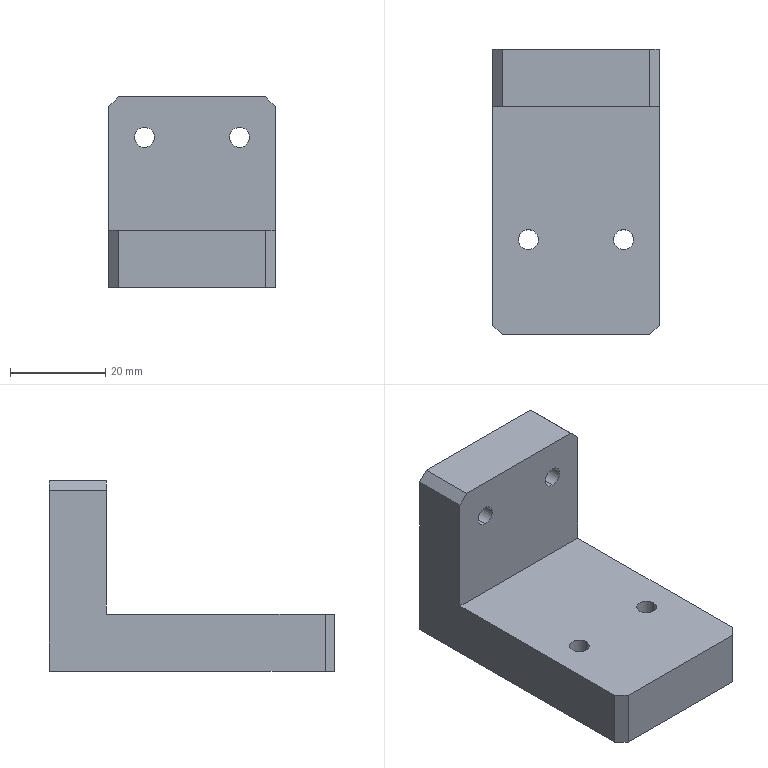Part | SolidWorks | features Chamfer 2, HoleWzd 2, Extrusion 1, ICE 1 | 1 solid | 28 faces | box 35 x 60 x 40 mm | volume 35844 mm3 | cylinder 12 | plane 12 | cone 4 | commonest cylinder face diameters 4.2 x12
STEP:
#1=CARTESIAN_POINT('',(-10.,17.6,4.4));
#2=VERTEX_POINT('',#1);
#3=CARTESIAN_POINT('',(-10.,17.6,8.6));
#4=VERTEX_POINT('',#3);
#5=CARTESIAN_POINT('',(-10.,17.6,6.5));
#6=DIRECTION('',(0.,1.,0.));
#7=DIRECTION('',(0.,0.,1.));
#8=AXIS2_PLACEMENT_3D('',#5,#6,#7);
#9=CIRCLE('',#8,2.1);
#10=EDGE_CURVE('',#2,#4,#9,.T.);
#11=ORIENTED_EDGE('',*,*,#10,.F.);
#12=CARTESIAN_POINT('',(-10.,30.,4.4));
#13=VERTEX_POINT('',#12);
#14=CARTESIAN_POINT('',(-10.,30.,4.4));
#15=DIRECTION('',(0.,1.,0.));
#16=VECTOR('',#15,1000.);
#17=LINE('',#14,#16);
#18=EDGE_CURVE('',#2,#13,#17,.T.);
#19=ORIENTED_EDGE('',*,*,#18,.T.);
#20=CARTESIAN_POINT('',(-10.,30.,8.6));
#21=VERTEX_POINT('',#20);
#22=CARTESIAN_POINT('',(-10.,30.,6.5));
#23=DIRECTION('',(0.,1.,0.));
#24=DIRECTION('',(0.,0.,1.));
#25=AXIS2_PLACEMENT_3D('',#22,#23,#24);
#26=CIRCLE('',#25,2.1);
#27=EDGE_CURVE('',#13,#21,#26,.T.);
#28=ORIENTED_EDGE('',*,*,#27,.T.);
#29=CARTESIAN_POINT('',(-10.,30.,8.6));
#30=DIRECTION('',(0.,1.,0.));
#31=VECTOR('',#30,1000.);
#32=LINE('',#29,#31);
#33=EDGE_CURVE('',#4,#21,#32,.T.);
#34=ORIENTED_EDGE('',*,*,#33,.F.);
#35=EDGE_LOOP('',(#11,#19,#28,#34));
#36=FACE_OUTER_BOUND('',#35,.T.);
#37=CARTESIAN_POINT('',(-10.,30.,6.5));
#38=DIRECTION('',(0.,1.,0.));
#39=DIRECTION('',(0.,0.,1.));
#40=AXIS2_PLACEMENT_3D('',#37,#38,#39);
#41=CYLINDRICAL_SURFACE('',#40,2.1);
#42=ADVANCED_FACE('',(#36),#41,.F.);
#43=CARTESIAN_POINT('',(-10.,16.338,6.5));
#44=VERTEX_POINT('',#43);
#45=CARTESIAN_POINT('',(-10.,17.6,8.6));
#46=DIRECTION('',(0.,0.515,0.8572));
#47=VECTOR('',#46,1000.);
#48=LINE('',#45,#47);
#49=EDGE_CURVE('',#44,#4,#48,.T.);
#50=ORIENTED_EDGE('',*,*,#49,.F.);
#51=CARTESIAN_POINT('',(-10.,17.6,4.4));
#52=DIRECTION('',(0.,0.515,-0.8572));
#53=VECTOR('',#52,1000.);
#54=LINE('',#51,#53);
#55=EDGE_CURVE('',#44,#2,#54,.T.);
#56=ORIENTED_EDGE('',*,*,#55,.T.);
#57=ORIENTED_EDGE('',*,*,#10,.T.);
#58=EDGE_LOOP('',(#50,#56,#57));
#59=FACE_OUTER_BOUND('',#58,.T.);
#60=CARTESIAN_POINT('',(-10.,17.6,6.5));
#61=DIRECTION('',(0.,1.,0.));
#62=DIRECTION('',(0.,0.,1.));
#63=AXIS2_PLACEMENT_3D('',#60,#61,#62);
#64=CONICAL_SURFACE('',#63,2.1,1.03);
#65=ADVANCED_FACE('',(#59),#64,.F.);
#66=CARTESIAN_POINT('',(10.,17.6,4.4));
#67=VERTEX_POINT('',#66);
#68=CARTESIAN_POINT('',(10.,17.6,8.6));
#69=VERTEX_POINT('',#68);
#70=CARTESIAN_POINT('',(10.,17.6,6.5));
#71=DIRECTION('',(0.,1.,0.));
#72=DIRECTION('',(0.,0.,1.));
#73=AXIS2_PLACEMENT_3D('',#70,#71,#72);
#74=CIRCLE('',#73,2.1);
#75=EDGE_CURVE('',#67,#69,#74,.T.);
#76=ORIENTED_EDGE('',*,*,#75,.F.);
#77=CARTESIAN_POINT('',(10.,30.,4.4));
#78=VERTEX_POINT('',#77);
#79=CARTESIAN_POINT('',(10.,30.,4.4));
#80=DIRECTION('',(0.,1.,0.));
#81=VECTOR('',#80,1000.);
#82=LINE('',#79,#81);
#83=EDGE_CURVE('',#67,#78,#82,.T.);
#84=ORIENTED_EDGE('',*,*,#83,.T.);
#85=CARTESIAN_POINT('',(10.,30.,8.6));
#86=VERTEX_POINT('',#85);
#87=CARTESIAN_POINT('',(10.,30.,6.5));
#88=DIRECTION('',(0.,1.,0.));
#89=DIRECTION('',(0.,0.,1.));
#90=AXIS2_PLACEMENT_3D('',#87,#88,#89);
#91=CIRCLE('',#90,2.1);
#92=EDGE_CURVE('',#78,#86,#91,.T.);
#93=ORIENTED_EDGE('',*,*,#92,.T.);
#94=CARTESIAN_POINT('',(10.,30.,8.6));
#95=DIRECTION('',(0.,1.,0.));
#96=VECTOR('',#95,1000.);
#97=LINE('',#94,#96);
#98=EDGE_CURVE('',#69,#86,#97,.T.);
#99=ORIENTED_EDGE('',*,*,#98,.F.);
#100=EDGE_LOOP('',(#76,#84,#93,#99));
#101=FACE_OUTER_BOUND('',#100,.T.);
#102=CARTESIAN_POINT('',(10.,30.,6.5));
#103=DIRECTION('',(0.,1.,0.));
#104=DIRECTION('',(0.,0.,1.));
#105=AXIS2_PLACEMENT_3D('',#102,#103,#104);
#106=CYLINDRICAL_SURFACE('',#105,2.1);
#107=ADVANCED_FACE('',(#101),#106,.F.);
#108=CARTESIAN_POINT('',(10.,16.338,6.5));
#109=VERTEX_POINT('',#108);
#110=CARTESIAN_POINT('',(10.,17.6,8.6));
#111=DIRECTION('',(0.,0.515,0.8572));
#112=VECTOR('',#111,1000.);
#113=LINE('',#110,#112);
#114=EDGE_CURVE('',#109,#69,#113,.T.);
#115=ORIENTED_EDGE('',*,*,#114,.F.);
#116=CARTESIAN_POINT('',(10.,17.6,4.4));
#117=DIRECTION('',(0.,0.515,-0.8572));
#118=VECTOR('',#117,1000.);
#119=LINE('',#116,#118);
#120=EDGE_CURVE('',#109,#67,#119,.T.);
#121=ORIENTED_EDGE('',*,*,#120,.T.);
#122=ORIENTED_EDGE('',*,*,#75,.T.);
#123=EDGE_LOOP('',(#115,#121,#122));
#124=FACE_OUTER_BOUND('',#123,.T.);
#125=CARTESIAN_POINT('',(10.,17.6,6.5));
#126=DIRECTION('',(0.,1.,0.));
#127=DIRECTION('',(0.,0.,1.));
#128=AXIS2_PLACEMENT_3D('',#125,#126,#127);
#129=CONICAL_SURFACE('',#128,2.1,1.03);
#130=ADVANCED_FACE('',(#124),#129,.F.);
#131=CARTESIAN_POINT('',(-10.,18.,33.6));
#132=VERTEX_POINT('',#131);
#133=CARTESIAN_POINT('',(-10.,18.,29.4));
#134=VERTEX_POINT('',#133);
#135=CARTESIAN_POINT('',(-10.,18.,31.5));
#136=DIRECTION('',(0.,-1.,0.));
#137=DIRECTION('',(0.,0.,-1.));
#138=AXIS2_PLACEMENT_3D('',#135,#136,#137);
#139=CIRCLE('',#138,2.1);
#140=EDGE_CURVE('',#132,#134,#139,.T.);
#141=ORIENTED_EDGE('',*,*,#140,.T.);
#142=CARTESIAN_POINT('',(-10.,30.,29.4));
#143=VERTEX_POINT('',#142);
#144=CARTESIAN_POINT('',(-10.,30.,29.4));
#145=DIRECTION('',(0.,1.,0.));
#146=VECTOR('',#145,1000.);
#147=LINE('',#144,#146);
#148=EDGE_CURVE('',#134,#143,#147,.T.);
#149=ORIENTED_EDGE('',*,*,#148,.T.);
#150=CARTESIAN_POINT('',(-10.,30.,33.6));
#151=VERTEX_POINT('',#150);
#152=CARTESIAN_POINT('',(-10.,30.,31.5));
#153=DIRECTION('',(0.,1.,0.));
#154=DIRECTION('',(0.,0.,1.));
#155=AXIS2_PLACEMENT_3D('',#152,#153,#154);
#156=CIRCLE('',#155,2.1);
#157=EDGE_CURVE('',#143,#151,#156,.T.);
#158=ORIENTED_EDGE('',*,*,#157,.T.);
#159=CARTESIAN_POINT('',(-10.,30.,33.6));
#160=DIRECTION('',(0.,1.,0.));
#161=VECTOR('',#160,1000.);
#162=LINE('',#159,#161);
#163=EDGE_CURVE('',#132,#151,#162,.T.);
#164=ORIENTED_EDGE('',*,*,#163,.F.);
#165=EDGE_LOOP('',(#141,#149,#158,#164));
#166=FACE_OUTER_BOUND('',#165,.T.);
#167=CARTESIAN_POINT('',(-10.,30.,31.5));
#168=DIRECTION('',(0.,1.,0.));
#169=DIRECTION('',(0.,0.,1.));
#170=AXIS2_PLACEMENT_3D('',#167,#168,#169);
#171=CYLINDRICAL_SURFACE('',#170,2.1);
#172=ADVANCED_FACE('',(#166),#171,.F.);
#173=CARTESIAN_POINT('',(10.,18.,33.6));
#174=VERTEX_POINT('',#173);
#175=CARTESIAN_POINT('',(10.,18.,29.4));
#176=VERTEX_POINT('',#175);
#177=CARTESIAN_POINT('',(10.,18.,31.5));
#178=DIRECTION('',(0.,-1.,0.));
#179=DIRECTION('',(0.,0.,-1.));
#180=AXIS2_PLACEMENT_3D('',#177,#178,#179);
#181=CIRCLE('',#180,2.1);
#182=EDGE_CURVE('',#174,#176,#181,.T.);
#183=ORIENTED_EDGE('',*,*,#182,.T.);
#184=CARTESIAN_POINT('',(10.,30.,29.4));
#185=VERTEX_POINT('',#184);
#186=CARTESIAN_POINT('',(10.,30.,29.4));
#187=DIRECTION('',(0.,1.,0.));
#188=VECTOR('',#187,1000.);
#189=LINE('',#186,#188);
#190=EDGE_CURVE('',#176,#185,#189,.T.);
#191=ORIENTED_EDGE('',*,*,#190,.T.);
#192=CARTESIAN_POINT('',(10.,30.,33.6));
#193=VERTEX_POINT('',#192);
#194=CARTESIAN_POINT('',(10.,30.,31.5));
#195=DIRECTION('',(0.,1.,0.));
#196=DIRECTION('',(0.,0.,1.));
#197=AXIS2_PLACEMENT_3D('',#194,#195,#196);
#198=CIRCLE('',#197,2.1);
#199=EDGE_CURVE('',#185,#193,#198,.T.);
#200=ORIENTED_EDGE('',*,*,#199,.T.);
#201=CARTESIAN_POINT('',(10.,30.,33.6));
#202=DIRECTION('',(0.,1.,0.));
#203=VECTOR('',#202,1000.);
#204=LINE('',#201,#203);
#205=EDGE_CURVE('',#174,#193,#204,.T.);
#206=ORIENTED_EDGE('',*,*,#205,.F.);
#207=EDGE_LOOP('',(#183,#191,#200,#206));
#208=FACE_OUTER_BOUND('',#207,.T.);
#209=CARTESIAN_POINT('',(10.,30.,31.5));
#210=DIRECTION('',(0.,1.,0.));
#211=DIRECTION('',(0.,0.,1.));
#212=AXIS2_PLACEMENT_3D('',#209,#210,#211);
#213=CYLINDRICAL_SURFACE('',#212,2.1);
#214=ADVANCED_FACE('',(#208),#213,.F.);
#215=CARTESIAN_POINT('',(12.1,-10.,12.));
#216=VERTEX_POINT('',#215);
#217=CARTESIAN_POINT('',(7.9,-10.,12.));
#218=VERTEX_POINT('',#217);
#219=CARTESIAN_POINT('',(10.,-10.,12.));
#220=DIRECTION('',(0.,0.,-1.));
#221=DIRECTION('',(-1.,0.,0.));
#222=AXIS2_PLACEMENT_3D('',#219,#220,#221);
#223=CIRCLE('',#222,2.1);
#224=EDGE_CURVE('',#216,#218,#223,.T.);
#225=ORIENTED_EDGE('',*,*,#224,.F.);
#226=CARTESIAN_POINT('',(12.1,-10.,0.));
#227=VERTEX_POINT('',#226);
#228=CARTESIAN_POINT('',(12.1,-10.,0.));
#229=DIRECTION('',(0.,0.,-1.));
#230=VECTOR('',#229,1000.);
#231=LINE('',#228,#230);
#232=EDGE_CURVE('',#216,#227,#231,.T.);
#233=ORIENTED_EDGE('',*,*,#232,.T.);
#234=CARTESIAN_POINT('',(7.9,-10.,0.));
#235=VERTEX_POINT('',#234);
#236=CARTESIAN_POINT('',(10.,-10.,0.));
#237=DIRECTION('',(0.,0.,-1.));
#238=DIRECTION('',(-1.,0.,0.));
#239=AXIS2_PLACEMENT_3D('',#236,#237,#238);
#240=CIRCLE('',#239,2.1);
#241=EDGE_CURVE('',#227,#235,#240,.T.);
#242=ORIENTED_EDGE('',*,*,#241,.T.);
#243=CARTESIAN_POINT('',(7.9,-10.,0.));
#244=DIRECTION('',(0.,0.,-1.));
#245=VECTOR('',#244,1000.);
#246=LINE('',#243,#245);
#247=EDGE_CURVE('',#218,#235,#246,.T.);
#248=ORIENTED_EDGE('',*,*,#247,.F.);
#249=EDGE_LOOP('',(#225,#233,#242,#248));
#250=FACE_OUTER_BOUND('',#249,.T.);
#251=CARTESIAN_POINT('',(10.,-10.,0.));
#252=DIRECTION('',(0.,0.,-1.));
#253=DIRECTION('',(-1.,0.,0.));
#254=AXIS2_PLACEMENT_3D('',#251,#252,#253);
#255=CYLINDRICAL_SURFACE('',#254,2.1);
#256=ADVANCED_FACE('',(#250),#255,.F.);
#257=CARTESIAN_POINT('',(-7.9,-10.,12.));
#258=VERTEX_POINT('',#257);
#259=CARTESIAN_POINT('',(-12.1,-10.,12.));
#260=VERTEX_POINT('',#259);
#261=CARTESIAN_POINT('',(-10.,-10.,12.));
#262=DIRECTION('',(0.,0.,-1.));
#263=DIRECTION('',(-1.,0.,0.));
#264=AXIS2_PLACEMENT_3D('',#261,#262,#263);
#265=CIRCLE('',#264,2.1);
#266=EDGE_CURVE('',#258,#260,#265,.T.);
#267=ORIENTED_EDGE('',*,*,#266,.F.);
#268=CARTESIAN_POINT('',(-7.9,-10.,0.));
#269=VERTEX_POINT('',#268);
#270=CARTESIAN_POINT('',(-7.9,-10.,0.));
#271=DIRECTION('',(0.,0.,-1.));
#272=VECTOR('',#271,1000.);
#273=LINE('',#270,#272);
#274=EDGE_CURVE('',#258,#269,#273,.T.);
#275=ORIENTED_EDGE('',*,*,#274,.T.);
#276=CARTESIAN_POINT('',(-12.1,-10.,0.));
#277=VERTEX_POINT('',#276);
#278=CARTESIAN_POINT('',(-10.,-10.,0.));
#279=DIRECTION('',(0.,0.,-1.));
#280=DIRECTION('',(-1.,0.,0.));
#281=AXIS2_PLACEMENT_3D('',#278,#279,#280);
#282=CIRCLE('',#281,2.1);
#283=EDGE_CURVE('',#269,#277,#282,.T.);
#284=ORIENTED_EDGE('',*,*,#283,.T.);
#285=CARTESIAN_POINT('',(-12.1,-10.,0.));
#286=DIRECTION('',(0.,0.,-1.));
#287=VECTOR('',#286,1000.);
#288=LINE('',#285,#287);
#289=EDGE_CURVE('',#260,#277,#288,.T.);
#290=ORIENTED_EDGE('',*,*,#289,.F.);
#291=EDGE_LOOP('',(#267,#275,#284,#290));
#292=FACE_OUTER_BOUND('',#291,.T.);
#293=CARTESIAN_POINT('',(-10.,-10.,0.));
#294=DIRECTION('',(0.,0.,-1.));
#295=DIRECTION('',(-1.,0.,0.));
#296=AXIS2_PLACEMENT_3D('',#293,#294,#295);
#297=CYLINDRICAL_SURFACE('',#296,2.1);
#298=ADVANCED_FACE('',(#292),#297,.F.);
#299=CARTESIAN_POINT('',(-17.5,18.,12.));
#300=VERTEX_POINT('',#299);
#301=CARTESIAN_POINT('',(-17.5,18.,38.));
#302=VERTEX_POINT('',#301);
#303=CARTESIAN_POINT('',(-17.5,18.,12.));
#304=DIRECTION('',(0.,0.,1.));
#305=VECTOR('',#304,1000.);
#306=LINE('',#303,#305);
#307=EDGE_CURVE('',#300,#302,#306,.T.);
#308=ORIENTED_EDGE('',*,*,#307,.T.);
#309=CARTESIAN_POINT('',(-17.5,30.,38.));
#310=VERTEX_POINT('',#309);
#311=CARTESIAN_POINT('',(-17.5,-30.,38.));
#312=DIRECTION('',(0.,1.,0.));
#313=VECTOR('',#312,1000.);
#314=LINE('',#311,#313);
#315=EDGE_CURVE('',#302,#310,#314,.T.);
#316=ORIENTED_EDGE('',*,*,#315,.T.);
#317=CARTESIAN_POINT('',(-17.5,30.,0.));
#318=VERTEX_POINT('',#317);
#319=CARTESIAN_POINT('',(-17.5,30.,12.));
#320=DIRECTION('',(0.,0.,-1.));
#321=VECTOR('',#320,1000.);
#322=LINE('',#319,#321);
#323=EDGE_CURVE('',#310,#318,#322,.T.);
#324=ORIENTED_EDGE('',*,*,#323,.T.);
#325=CARTESIAN_POINT('',(-17.5,-28.,0.));
#326=VERTEX_POINT('',#325);
#327=CARTESIAN_POINT('',(-17.5,-30.,0.));
#328=DIRECTION('',(0.,1.,0.));
#329=VECTOR('',#328,1000.);
#330=LINE('',#327,#329);
#331=EDGE_CURVE('',#326,#318,#330,.T.);
#332=ORIENTED_EDGE('',*,*,#331,.F.);
#333=CARTESIAN_POINT('',(-17.5,-28.,12.));
#334=VERTEX_POINT('',#333);
#335=CARTESIAN_POINT('',(-17.5,-28.,12.));
#336=DIRECTION('',(0.,0.,1.));
#337=VECTOR('',#336,1000.);
#338=LINE('',#335,#337);
#339=EDGE_CURVE('',#326,#334,#338,.T.);
#340=ORIENTED_EDGE('',*,*,#339,.T.);
#341=CARTESIAN_POINT('',(-17.5,-30.,12.));
#342=DIRECTION('',(0.,1.,0.));
#343=VECTOR('',#342,1000.);
#344=LINE('',#341,#343);
#345=EDGE_CURVE('',#334,#300,#344,.T.);
#346=ORIENTED_EDGE('',*,*,#345,.T.);
#347=EDGE_LOOP('',(#308,#316,#324,#332,#340,#346));
#348=FACE_OUTER_BOUND('',#347,.T.);
#349=CARTESIAN_POINT('',(-17.5,-30.,12.));
#350=DIRECTION('',(-1.,0.,0.));
#351=DIRECTION('',(0.,0.,1.));
#352=AXIS2_PLACEMENT_3D('',#349,#350,#351);
#353=PLANE('',#352);
#354=ADVANCED_FACE('',(#348),#353,.T.);
#355=CARTESIAN_POINT('',(-15.5,-30.,0.));
#356=VERTEX_POINT('',#355);
#357=CARTESIAN_POINT('',(15.5,-30.,0.));
#358=VERTEX_POINT('',#357);
#359=CARTESIAN_POINT('',(-17.5,-30.,0.));
#360=DIRECTION('',(1.,0.,0.));
#361=VECTOR('',#360,1000.);
#362=LINE('',#359,#361);
#363=EDGE_CURVE('',#356,#358,#362,.T.);
#364=ORIENTED_EDGE('',*,*,#363,.T.);
#365=CARTESIAN_POINT('',(15.5,-30.,12.));
#366=VERTEX_POINT('',#365);
#367=CARTESIAN_POINT('',(15.5,-30.,12.));
#368=DIRECTION('',(0.,0.,1.));
#369=VECTOR('',#368,1000.);
#370=LINE('',#367,#369);
#371=EDGE_CURVE('',#358,#366,#370,.T.);
#372=ORIENTED_EDGE('',*,*,#371,.T.);
#373=CARTESIAN_POINT('',(-15.5,-30.,12.));
#374=VERTEX_POINT('',#373);
#375=CARTESIAN_POINT('',(-17.5,-30.,12.));
#376=DIRECTION('',(1.,0.,0.));
#377=VECTOR('',#376,1000.);
#378=LINE('',#375,#377);
#379=EDGE_CURVE('',#374,#366,#378,.T.);
#380=ORIENTED_EDGE('',*,*,#379,.F.);
#381=CARTESIAN_POINT('',(-15.5,-30.,0.));
#382=DIRECTION('',(0.,0.,-1.));
#383=VECTOR('',#382,1000.);
#384=LINE('',#381,#383);
#385=EDGE_CURVE('',#374,#356,#384,.T.);
#386=ORIENTED_EDGE('',*,*,#385,.T.);
#387=EDGE_LOOP('',(#364,#372,#380,#386));
#388=FACE_OUTER_BOUND('',#387,.T.);
#389=CARTESIAN_POINT('',(-17.5,-30.,12.));
#390=DIRECTION('',(0.,1.,0.));
#391=DIRECTION('',(0.,0.,1.));
#392=AXIS2_PLACEMENT_3D('',#389,#390,#391);
#393=PLANE('',#392);
#394=ADVANCED_FACE('',(#388),#393,.F.);
#395=CARTESIAN_POINT('',(17.5,30.,38.));
#396=VERTEX_POINT('',#395);
#397=CARTESIAN_POINT('',(17.5,30.,0.));
#398=VERTEX_POINT('',#397);
#399=CARTESIAN_POINT('',(17.5,30.,12.));
#400=DIRECTION('',(0.,0.,-1.));
#401=VECTOR('',#400,1000.);
#402=LINE('',#399,#401);
#403=EDGE_CURVE('',#396,#398,#402,.T.);
#404=ORIENTED_EDGE('',*,*,#403,.F.);
#405=CARTESIAN_POINT('',(17.5,18.,38.));
#406=VERTEX_POINT('',#405);
#407=CARTESIAN_POINT('',(17.5,18.,38.));
#408=DIRECTION('',(0.,-1.,0.));
#409=VECTOR('',#408,1000.);
#410=LINE('',#407,#409);
#411=EDGE_CURVE('',#396,#406,#410,.T.);
#412=ORIENTED_EDGE('',*,*,#411,.T.);
#413=CARTESIAN_POINT('',(17.5,18.,12.));
#414=VERTEX_POINT('',#413);
#415=CARTESIAN_POINT('',(17.5,18.,12.));
#416=DIRECTION('',(0.,0.,-1.));
#417=VECTOR('',#416,1000.);
#418=LINE('',#415,#417);
#419=EDGE_CURVE('',#406,#414,#418,.T.);
#420=ORIENTED_EDGE('',*,*,#419,.T.);
#421=CARTESIAN_POINT('',(17.5,-28.,12.));
#422=VERTEX_POINT('',#421);
#423=CARTESIAN_POINT('',(17.5,-30.,12.));
#424=DIRECTION('',(0.,1.,0.));
#425=VECTOR('',#424,1000.);
#426=LINE('',#423,#425);
#427=EDGE_CURVE('',#422,#414,#426,.T.);
#428=ORIENTED_EDGE('',*,*,#427,.F.);
#429=CARTESIAN_POINT('',(17.5,-28.,0.));
#430=VERTEX_POINT('',#429);
#431=CARTESIAN_POINT('',(17.5,-28.,12.));
#432=DIRECTION('',(0.,0.,-1.));
#433=VECTOR('',#432,1000.);
#434=LINE('',#431,#433);
#435=EDGE_CURVE('',#422,#430,#434,.T.);
#436=ORIENTED_EDGE('',*,*,#435,.T.);
#437=CARTESIAN_POINT('',(17.5,-30.,0.));
#438=DIRECTION('',(0.,1.,0.));
#439=VECTOR('',#438,1000.);
#440=LINE('',#437,#439);
#441=EDGE_CURVE('',#430,#398,#440,.T.);
#442=ORIENTED_EDGE('',*,*,#441,.T.);
#443=EDGE_LOOP('',(#404,#412,#420,#428,#436,#442));
#444=FACE_OUTER_BOUND('',#443,.T.);
#445=CARTESIAN_POINT('',(17.5,-30.,12.));
#446=DIRECTION('',(-1.,0.,0.));
#447=DIRECTION('',(0.,0.,1.));
#448=AXIS2_PLACEMENT_3D('',#445,#446,#447);
#449=PLANE('',#448);
#450=ADVANCED_FACE('',(#444),#449,.F.);
#451=CARTESIAN_POINT('',(-10.,30.,6.5));
#452=DIRECTION('',(0.,1.,0.));
#453=DIRECTION('',(0.,0.,1.));
#454=AXIS2_PLACEMENT_3D('',#451,#452,#453);
#455=CIRCLE('',#454,2.1);
#456=EDGE_CURVE('',#21,#13,#455,.T.);
#457=ORIENTED_EDGE('',*,*,#456,.F.);
#458=ORIENTED_EDGE('',*,*,#27,.F.);
#459=EDGE_LOOP('',(#457,#458));
#460=FACE_BOUND('',#459,.T.);
#461=CARTESIAN_POINT('',(10.,30.,6.5));
#462=DIRECTION('',(0.,1.,0.));
#463=DIRECTION('',(0.,0.,1.));
#464=AXIS2_PLACEMENT_3D('',#461,#462,#463);
#465=CIRCLE('',#464,2.1);
#466=EDGE_CURVE('',#86,#78,#465,.T.);
#467=ORIENTED_EDGE('',*,*,#466,.F.);
#468=ORIENTED_EDGE('',*,*,#92,.F.);
#469=EDGE_LOOP('',(#467,#468));
#470=FACE_BOUND('',#469,.T.);
#471=CARTESIAN_POINT('',(-10.,30.,31.5));
#472=DIRECTION('',(0.,1.,0.));
#473=DIRECTION('',(0.,0.,1.));
#474=AXIS2_PLACEMENT_3D('',#471,#472,#473);
#475=CIRCLE('',#474,2.1);
#476=EDGE_CURVE('',#151,#143,#475,.T.);
#477=ORIENTED_EDGE('',*,*,#476,.F.);
#478=ORIENTED_EDGE('',*,*,#157,.F.);
#479=EDGE_LOOP('',(#477,#478));
#480=FACE_BOUND('',#479,.T.);
#481=CARTESIAN_POINT('',(10.,30.,31.5));
#482=DIRECTION('',(0.,1.,0.));
#483=DIRECTION('',(0.,0.,1.));
#484=AXIS2_PLACEMENT_3D('',#481,#482,#483);
#485=CIRCLE('',#484,2.1);
#486=EDGE_CURVE('',#193,#185,#485,.T.);
#487=ORIENTED_EDGE('',*,*,#486,.F.);
#488=ORIENTED_EDGE('',*,*,#199,.F.);
#489=EDGE_LOOP('',(#487,#488));
#490=FACE_BOUND('',#489,.T.);
#491=CARTESIAN_POINT('',(15.5,30.,40.));
#492=VERTEX_POINT('',#491);
#493=CARTESIAN_POINT('',(-15.5,30.,40.));
#494=VERTEX_POINT('',#493);
#495=CARTESIAN_POINT('',(47.963,30.,40.));
#496=DIRECTION('',(-1.,0.,0.));
#497=VECTOR('',#496,1000.);
#498=LINE('',#495,#497);
#499=EDGE_CURVE('',#492,#494,#498,.T.);
#500=ORIENTED_EDGE('',*,*,#499,.F.);
#501=CARTESIAN_POINT('',(13.,30.,42.5));
#502=DIRECTION('',(0.7071,0.,-0.7071));
#503=VECTOR('',#502,1000.);
#504=LINE('',#501,#503);
#505=EDGE_CURVE('',#492,#396,#504,.T.);
#506=ORIENTED_EDGE('',*,*,#505,.T.);
#507=ORIENTED_EDGE('',*,*,#403,.T.);
#508=CARTESIAN_POINT('',(-17.5,30.,0.));
#509=DIRECTION('',(1.,0.,0.));
#510=VECTOR('',#509,1000.);
#511=LINE('',#508,#510);
#512=EDGE_CURVE('',#318,#398,#511,.T.);
#513=ORIENTED_EDGE('',*,*,#512,.F.);
#514=ORIENTED_EDGE('',*,*,#323,.F.);
#515=CARTESIAN_POINT('',(-30.5,30.,25.));
#516=DIRECTION('',(0.7071,0.,0.7071));
#517=VECTOR('',#516,1000.);
#518=LINE('',#515,#517);
#519=EDGE_CURVE('',#310,#494,#518,.T.);
#520=ORIENTED_EDGE('',*,*,#519,.T.);
#521=EDGE_LOOP('',(#500,#506,#507,#513,#514,#520));
#522=FACE_OUTER_BOUND('',#521,.T.);
#523=CARTESIAN_POINT('',(-17.5,30.,12.));
#524=DIRECTION('',(0.,1.,0.));
#525=DIRECTION('',(0.,0.,1.));
#526=AXIS2_PLACEMENT_3D('',#523,#524,#525);
#527=PLANE('',#526);
#528=ADVANCED_FACE('',(#460,#470,#480,#490,#522),#527,.T.);
#529=CARTESIAN_POINT('',(10.,-10.,12.));
#530=DIRECTION('',(0.,0.,-1.));
#531=DIRECTION('',(-1.,0.,0.));
#532=AXIS2_PLACEMENT_3D('',#529,#530,#531);
#533=CIRCLE('',#532,2.1);
#534=EDGE_CURVE('',#218,#216,#533,.T.);
#535=ORIENTED_EDGE('',*,*,#534,.T.);
#536=ORIENTED_EDGE('',*,*,#224,.T.);
#537=EDGE_LOOP('',(#535,#536));
#538=FACE_BOUND('',#537,.T.);
#539=CARTESIAN_POINT('',(-10.,-10.,12.));
#540=DIRECTION('',(0.,0.,-1.));
#541=DIRECTION('',(-1.,0.,0.));
#542=AXIS2_PLACEMENT_3D('',#539,#540,#541);
#543=CIRCLE('',#542,2.1);
#544=EDGE_CURVE('',#260,#258,#543,.T.);
#545=ORIENTED_EDGE('',*,*,#544,.T.);
#546=ORIENTED_EDGE('',*,*,#266,.T.);
#547=EDGE_LOOP('',(#545,#546));
#548=FACE_BOUND('',#547,.T.);
#549=ORIENTED_EDGE('',*,*,#427,.T.);
#550=CARTESIAN_POINT('',(47.963,18.,12.));
#551=DIRECTION('',(-1.,0.,0.));
#552=VECTOR('',#551,1000.);
#553=LINE('',#550,#552);
#554=EDGE_CURVE('',#414,#300,#553,.T.);
#555=ORIENTED_EDGE('',*,*,#554,.T.);
#556=ORIENTED_EDGE('',*,*,#345,.F.);
#557=CARTESIAN_POINT('',(-15.5,-30.,12.));
#558=DIRECTION('',(0.7071,-0.7071,0.));
#559=VECTOR('',#558,1000.);
#560=LINE('',#557,#559);
#561=EDGE_CURVE('',#334,#374,#560,.T.);
#562=ORIENTED_EDGE('',*,*,#561,.T.);
#563=ORIENTED_EDGE('',*,*,#379,.T.);
#564=CARTESIAN_POINT('',(17.5,-28.,12.));
#565=DIRECTION('',(0.7071,0.7071,0.));
#566=VECTOR('',#565,1000.);
#567=LINE('',#564,#566);
#568=EDGE_CURVE('',#366,#422,#567,.T.);
#569=ORIENTED_EDGE('',*,*,#568,.T.);
#570=EDGE_LOOP('',(#549,#555,#556,#562,#563,#569));
#571=FACE_OUTER_BOUND('',#570,.T.);
#572=CARTESIAN_POINT('',(0.,0.,12.));
#573=DIRECTION('',(0.,0.,-1.));
#574=DIRECTION('',(-1.,0.,0.));
#575=AXIS2_PLACEMENT_3D('',#572,#573,#574);
#576=PLANE('',#575);
#577=ADVANCED_FACE('',(#538,#548,#571),#576,.F.);
#578=CARTESIAN_POINT('',(10.,-10.,0.));
#579=DIRECTION('',(0.,0.,-1.));
#580=DIRECTION('',(-1.,0.,0.));
#581=AXIS2_PLACEMENT_3D('',#578,#579,#580);
#582=CIRCLE('',#581,2.1);
#583=EDGE_CURVE('',#235,#227,#582,.T.);
#584=ORIENTED_EDGE('',*,*,#583,.F.);
#585=ORIENTED_EDGE('',*,*,#241,.F.);
#586=EDGE_LOOP('',(#584,#585));
#587=FACE_BOUND('',#586,.T.);
#588=CARTESIAN_POINT('',(-10.,-10.,0.));
#589=DIRECTION('',(0.,0.,-1.));
#590=DIRECTION('',(-1.,0.,0.));
#591=AXIS2_PLACEMENT_3D('',#588,#589,#590);
#592=CIRCLE('',#591,2.1);
#593=EDGE_CURVE('',#277,#269,#592,.T.);
#594=ORIENTED_EDGE('',*,*,#593,.F.);
#595=ORIENTED_EDGE('',*,*,#283,.F.);
#596=EDGE_LOOP('',(#594,#595));
#597=FACE_BOUND('',#596,.T.);
#598=ORIENTED_EDGE('',*,*,#441,.F.);
#599=CARTESIAN_POINT('',(22.75,-22.75,0.));
#600=DIRECTION('',(-0.7071,-0.7071,0.));
#601=VECTOR('',#600,1000.);
#602=LINE('',#599,#601);
#603=EDGE_CURVE('',#430,#358,#602,.T.);
#604=ORIENTED_EDGE('',*,*,#603,.T.);
#605=ORIENTED_EDGE('',*,*,#363,.F.);
#606=CARTESIAN_POINT('',(-22.75,-22.75,0.));
#607=DIRECTION('',(-0.7071,0.7071,0.));
#608=VECTOR('',#607,1000.);
#609=LINE('',#606,#608);
#610=EDGE_CURVE('',#356,#326,#609,.T.);
#611=ORIENTED_EDGE('',*,*,#610,.T.);
#612=ORIENTED_EDGE('',*,*,#331,.T.);
#613=ORIENTED_EDGE('',*,*,#512,.T.);
#614=EDGE_LOOP('',(#598,#604,#605,#611,#612,#613));
#615=FACE_OUTER_BOUND('',#614,.T.);
#616=CARTESIAN_POINT('',(0.,0.,0.));
#617=DIRECTION('',(0.,0.,-1.));
#618=DIRECTION('',(-1.,0.,0.));
#619=AXIS2_PLACEMENT_3D('',#616,#617,#618);
#620=PLANE('',#619);
#621=ADVANCED_FACE('',(#587,#597,#615),#620,.T.);
#622=ORIENTED_EDGE('',*,*,#568,.F.);
#623=ORIENTED_EDGE('',*,*,#371,.F.);
#624=ORIENTED_EDGE('',*,*,#603,.F.);
#625=ORIENTED_EDGE('',*,*,#435,.F.);
#626=EDGE_LOOP('',(#622,#623,#624,#625));
#627=FACE_OUTER_BOUND('',#626,.T.);
#628=CARTESIAN_POINT('',(17.5,-28.,12.));
#629=DIRECTION('',(-0.7071,0.7071,0.));
#630=DIRECTION('',(0.,0.,-1.));
#631=AXIS2_PLACEMENT_3D('',#628,#629,#630);
#632=PLANE('',#631);
#633=ADVANCED_FACE('',(#627),#632,.F.);
#634=ORIENTED_EDGE('',*,*,#561,.F.);
#635=ORIENTED_EDGE('',*,*,#339,.F.);
#636=ORIENTED_EDGE('',*,*,#610,.F.);
#637=ORIENTED_EDGE('',*,*,#385,.F.);
#638=EDGE_LOOP('',(#634,#635,#636,#637));
#639=FACE_OUTER_BOUND('',#638,.T.);
#640=CARTESIAN_POINT('',(-15.5,-30.,12.));
#641=DIRECTION('',(-0.7071,-0.7071,0.));
#642=DIRECTION('',(0.,0.,1.));
#643=AXIS2_PLACEMENT_3D('',#640,#641,#642);
#644=PLANE('',#643);
#645=ADVANCED_FACE('',(#639),#644,.T.);
#646=CARTESIAN_POINT('',(15.5,18.,40.));
#647=VERTEX_POINT('',#646);
#648=CARTESIAN_POINT('',(-15.5,18.,40.));
#649=VERTEX_POINT('',#648);
#650=CARTESIAN_POINT('',(47.963,18.,40.));
#651=DIRECTION('',(-1.,0.,0.));
#652=VECTOR('',#651,1000.);
#653=LINE('',#650,#652);
#654=EDGE_CURVE('',#647,#649,#653,.T.);
#655=ORIENTED_EDGE('',*,*,#654,.F.);
#656=CARTESIAN_POINT('',(15.5,30.,40.));
#657=DIRECTION('',(0.,1.,0.));
#658=VECTOR('',#657,1000.);
#659=LINE('',#656,#658);
#660=EDGE_CURVE('',#647,#492,#659,.T.);
#661=ORIENTED_EDGE('',*,*,#660,.T.);
#662=ORIENTED_EDGE('',*,*,#499,.T.);
#663=CARTESIAN_POINT('',(-15.5,30.,40.));
#664=DIRECTION('',(0.,-1.,0.));
#665=VECTOR('',#664,1000.);
#666=LINE('',#663,#665);
#667=EDGE_CURVE('',#494,#649,#666,.T.);
#668=ORIENTED_EDGE('',*,*,#667,.T.);
#669=EDGE_LOOP('',(#655,#661,#662,#668));
#670=FACE_OUTER_BOUND('',#669,.T.);
#671=CARTESIAN_POINT('',(47.963,30.,40.));
#672=DIRECTION('',(0.,0.,1.));
#673=DIRECTION('',(0.,-1.,0.));
#674=AXIS2_PLACEMENT_3D('',#671,#672,#673);
#675=PLANE('',#674);
#676=ADVANCED_FACE('',(#670),#675,.T.);
#677=ORIENTED_EDGE('',*,*,#140,.F.);
#678=CARTESIAN_POINT('',(-10.,18.,31.5));
#679=DIRECTION('',(0.,-1.,0.));
#680=DIRECTION('',(0.,0.,-1.));
#681=AXIS2_PLACEMENT_3D('',#678,#679,#680);
#682=CIRCLE('',#681,2.1);
#683=EDGE_CURVE('',#134,#132,#682,.T.);
#684=ORIENTED_EDGE('',*,*,#683,.F.);
#685=EDGE_LOOP('',(#677,#684));
#686=FACE_BOUND('',#685,.T.);
#687=ORIENTED_EDGE('',*,*,#182,.F.);
#688=CARTESIAN_POINT('',(10.,18.,31.5));
#689=DIRECTION('',(0.,-1.,0.));
#690=DIRECTION('',(0.,0.,-1.));
#691=AXIS2_PLACEMENT_3D('',#688,#689,#690);
#692=CIRCLE('',#691,2.1);
#693=EDGE_CURVE('',#176,#174,#692,.T.);
#694=ORIENTED_EDGE('',*,*,#693,.F.);
#695=EDGE_LOOP('',(#687,#694));
#696=FACE_BOUND('',#695,.T.);
#697=ORIENTED_EDGE('',*,*,#419,.F.);
#698=CARTESIAN_POINT('',(45.732,18.,9.768));
#699=DIRECTION('',(-0.7071,0.,0.7071));
#700=VECTOR('',#699,1000.);
#701=LINE('',#698,#700);
#702=EDGE_CURVE('',#406,#647,#701,.T.);
#703=ORIENTED_EDGE('',*,*,#702,.T.);
#704=ORIENTED_EDGE('',*,*,#654,.T.);
#705=CARTESIAN_POINT('',(2.232,18.,57.732));
#706=DIRECTION('',(-0.7071,0.,-0.7071));
#707=VECTOR('',#706,1000.);
#708=LINE('',#705,#707);
#709=EDGE_CURVE('',#649,#302,#708,.T.);
#710=ORIENTED_EDGE('',*,*,#709,.T.);
#711=ORIENTED_EDGE('',*,*,#307,.F.);
#712=ORIENTED_EDGE('',*,*,#554,.F.);
#713=EDGE_LOOP('',(#697,#703,#704,#710,#711,#712));
#714=FACE_OUTER_BOUND('',#713,.T.);
#715=CARTESIAN_POINT('',(47.963,18.,12.));
#716=DIRECTION('',(0.,-1.,0.));
#717=DIRECTION('',(0.,0.,-1.));
#718=AXIS2_PLACEMENT_3D('',#715,#716,#717);
#719=PLANE('',#718);
#720=ADVANCED_FACE('',(#686,#696,#714),#719,.T.);
#721=ORIENTED_EDGE('',*,*,#274,.F.);
#722=ORIENTED_EDGE('',*,*,#544,.F.);
#723=ORIENTED_EDGE('',*,*,#289,.T.);
#724=ORIENTED_EDGE('',*,*,#593,.T.);
#725=EDGE_LOOP('',(#721,#722,#723,#724));
#726=FACE_OUTER_BOUND('',#725,.T.);
#727=CARTESIAN_POINT('',(-10.,-10.,0.));
#728=DIRECTION('',(0.,0.,-1.));
#729=DIRECTION('',(-1.,0.,0.));
#730=AXIS2_PLACEMENT_3D('',#727,#728,#729);
#731=CYLINDRICAL_SURFACE('',#730,2.1);
#732=ADVANCED_FACE('',(#726),#731,.F.);
#733=ORIENTED_EDGE('',*,*,#232,.F.);
#734=ORIENTED_EDGE('',*,*,#534,.F.);
#735=ORIENTED_EDGE('',*,*,#247,.T.);
#736=ORIENTED_EDGE('',*,*,#583,.T.);
#737=EDGE_LOOP('',(#733,#734,#735,#736));
#738=FACE_OUTER_BOUND('',#737,.T.);
#739=CARTESIAN_POINT('',(10.,-10.,0.));
#740=DIRECTION('',(0.,0.,-1.));
#741=DIRECTION('',(-1.,0.,0.));
#742=AXIS2_PLACEMENT_3D('',#739,#740,#741);
#743=CYLINDRICAL_SURFACE('',#742,2.1);
#744=ADVANCED_FACE('',(#738),#743,.F.);
#745=ORIENTED_EDGE('',*,*,#505,.F.);
#746=ORIENTED_EDGE('',*,*,#660,.F.);
#747=ORIENTED_EDGE('',*,*,#702,.F.);
#748=ORIENTED_EDGE('',*,*,#411,.F.);
#749=EDGE_LOOP('',(#745,#746,#747,#748));
#750=FACE_OUTER_BOUND('',#749,.T.);
#751=CARTESIAN_POINT('',(17.5,-30.,38.));
#752=DIRECTION('',(0.7071,0.,0.7071));
#753=DIRECTION('',(0.,1.,0.));
#754=AXIS2_PLACEMENT_3D('',#751,#752,#753);
#755=PLANE('',#754);
#756=ADVANCED_FACE('',(#750),#755,.T.);
#757=ORIENTED_EDGE('',*,*,#709,.F.);
#758=ORIENTED_EDGE('',*,*,#667,.F.);
#759=ORIENTED_EDGE('',*,*,#519,.F.);
#760=ORIENTED_EDGE('',*,*,#315,.F.);
#761=EDGE_LOOP('',(#757,#758,#759,#760));
#762=FACE_OUTER_BOUND('',#761,.T.);
#763=CARTESIAN_POINT('',(-17.5,-30.,38.));
#764=DIRECTION('',(0.7071,0.,-0.7071));
#765=DIRECTION('',(0.,1.,0.));
#766=AXIS2_PLACEMENT_3D('',#763,#764,#765);
#767=PLANE('',#766);
#768=ADVANCED_FACE('',(#762),#767,.F.);
#769=ORIENTED_EDGE('',*,*,#190,.F.);
#770=ORIENTED_EDGE('',*,*,#693,.T.);
#771=ORIENTED_EDGE('',*,*,#205,.T.);
#772=ORIENTED_EDGE('',*,*,#486,.T.);
#773=EDGE_LOOP('',(#769,#770,#771,#772));
#774=FACE_OUTER_BOUND('',#773,.T.);
#775=CARTESIAN_POINT('',(10.,30.,31.5));
#776=DIRECTION('',(0.,1.,0.));
#777=DIRECTION('',(0.,0.,1.));
#778=AXIS2_PLACEMENT_3D('',#775,#776,#777);
#779=CYLINDRICAL_SURFACE('',#778,2.1);
#780=ADVANCED_FACE('',(#774),#779,.F.);
#781=ORIENTED_EDGE('',*,*,#148,.F.);
#782=ORIENTED_EDGE('',*,*,#683,.T.);
#783=ORIENTED_EDGE('',*,*,#163,.T.);
#784=ORIENTED_EDGE('',*,*,#476,.T.);
#785=EDGE_LOOP('',(#781,#782,#783,#784));
#786=FACE_OUTER_BOUND('',#785,.T.);
#787=CARTESIAN_POINT('',(-10.,30.,31.5));
#788=DIRECTION('',(0.,1.,0.));
#789=DIRECTION('',(0.,0.,1.));
#790=AXIS2_PLACEMENT_3D('',#787,#788,#789);
#791=CYLINDRICAL_SURFACE('',#790,2.1);
#792=ADVANCED_FACE('',(#786),#791,.F.);
#793=ORIENTED_EDGE('',*,*,#120,.F.);
#794=ORIENTED_EDGE('',*,*,#114,.T.);
#795=CARTESIAN_POINT('',(10.,17.6,6.5));
#796=DIRECTION('',(0.,1.,0.));
#797=DIRECTION('',(0.,0.,1.));
#798=AXIS2_PLACEMENT_3D('',#795,#796,#797);
#799=CIRCLE('',#798,2.1);
#800=EDGE_CURVE('',#69,#67,#799,.T.);
#801=ORIENTED_EDGE('',*,*,#800,.T.);
#802=EDGE_LOOP('',(#793,#794,#801));
#803=FACE_OUTER_BOUND('',#802,.T.);
#804=CARTESIAN_POINT('',(10.,17.6,6.5));
#805=DIRECTION('',(0.,1.,0.));
#806=DIRECTION('',(0.,0.,1.));
#807=AXIS2_PLACEMENT_3D('',#804,#805,#806);
#808=CONICAL_SURFACE('',#807,2.1,1.03);
#809=ADVANCED_FACE('',(#803),#808,.F.);
#810=ORIENTED_EDGE('',*,*,#83,.F.);
#811=ORIENTED_EDGE('',*,*,#800,.F.);
#812=ORIENTED_EDGE('',*,*,#98,.T.);
#813=ORIENTED_EDGE('',*,*,#466,.T.);
#814=EDGE_LOOP('',(#810,#811,#812,#813));
#815=FACE_OUTER_BOUND('',#814,.T.);
#816=CARTESIAN_POINT('',(10.,30.,6.5));
#817=DIRECTION('',(0.,1.,0.));
#818=DIRECTION('',(0.,0.,1.));
#819=AXIS2_PLACEMENT_3D('',#816,#817,#818);
#820=CYLINDRICAL_SURFACE('',#819,2.1);
#821=ADVANCED_FACE('',(#815),#820,.F.);
#822=ORIENTED_EDGE('',*,*,#55,.F.);
#823=ORIENTED_EDGE('',*,*,#49,.T.);
#824=CARTESIAN_POINT('',(-10.,17.6,6.5));
#825=DIRECTION('',(0.,1.,0.));
#826=DIRECTION('',(0.,0.,1.));
#827=AXIS2_PLACEMENT_3D('',#824,#825,#826);
#828=CIRCLE('',#827,2.1);
#829=EDGE_CURVE('',#4,#2,#828,.T.);
#830=ORIENTED_EDGE('',*,*,#829,.T.);
#831=EDGE_LOOP('',(#822,#823,#830));
#832=FACE_OUTER_BOUND('',#831,.T.);
#833=CARTESIAN_POINT('',(-10.,17.6,6.5));
#834=DIRECTION('',(0.,1.,0.));
#835=DIRECTION('',(0.,0.,1.));
#836=AXIS2_PLACEMENT_3D('',#833,#834,#835);
#837=CONICAL_SURFACE('',#836,2.1,1.03);
#838=ADVANCED_FACE('',(#832),#837,.F.);
#839=ORIENTED_EDGE('',*,*,#18,.F.);
#840=ORIENTED_EDGE('',*,*,#829,.F.);
#841=ORIENTED_EDGE('',*,*,#33,.T.);
#842=ORIENTED_EDGE('',*,*,#456,.T.);
#843=EDGE_LOOP('',(#839,#840,#841,#842));
#844=FACE_OUTER_BOUND('',#843,.T.);
#845=CARTESIAN_POINT('',(-10.,30.,6.5));
#846=DIRECTION('',(0.,1.,0.));
#847=DIRECTION('',(0.,0.,1.));
#848=AXIS2_PLACEMENT_3D('',#845,#846,#847);
#849=CYLINDRICAL_SURFACE('',#848,2.1);
#850=ADVANCED_FACE('',(#844),#849,.F.);
#851=CLOSED_SHELL('',(#42,#65,#107,#130,#172,#214,#256,#298,#354,#394,#450,#528,#577,#621,#633,#645,#676,#720,#732,#744,#756,#768,#780,#792,#809,#821,#838,#850));
#852=MANIFOLD_SOLID_BREP('',#851);
#853=CARTESIAN_POINT('',(0.,0.,0.));
#854=DIRECTION('',(0.,0.,1.));
#855=DIRECTION('',(1.,0.,0.));
#856=AXIS2_PLACEMENT_3D('',#853,#854,#855);
#857=(LENGTH_UNIT()NAMED_UNIT(*)SI_UNIT(.MILLI.,.METRE.));
#858=UNCERTAINTY_MEASURE_WITH_UNIT(LENGTH_MEASURE(0.00001),#857,'','');
#859=(NAMED_UNIT(*)PLANE_ANGLE_UNIT()SI_UNIT($,.RADIAN.));
#860=(NAMED_UNIT(*)SI_UNIT($,.STERADIAN.)SOLID_ANGLE_UNIT());
#861=(GEOMETRIC_REPRESENTATION_CONTEXT(3)GLOBAL_UNCERTAINTY_ASSIGNED_CONTEXT((#858))GLOBAL_UNIT_ASSIGNED_CONTEXT((#857,#859,#860))REPRESENTATION_CONTEXT('',''));
#862=ADVANCED_BREP_SHAPE_REPRESENTATION('',(#852,#856),#861);